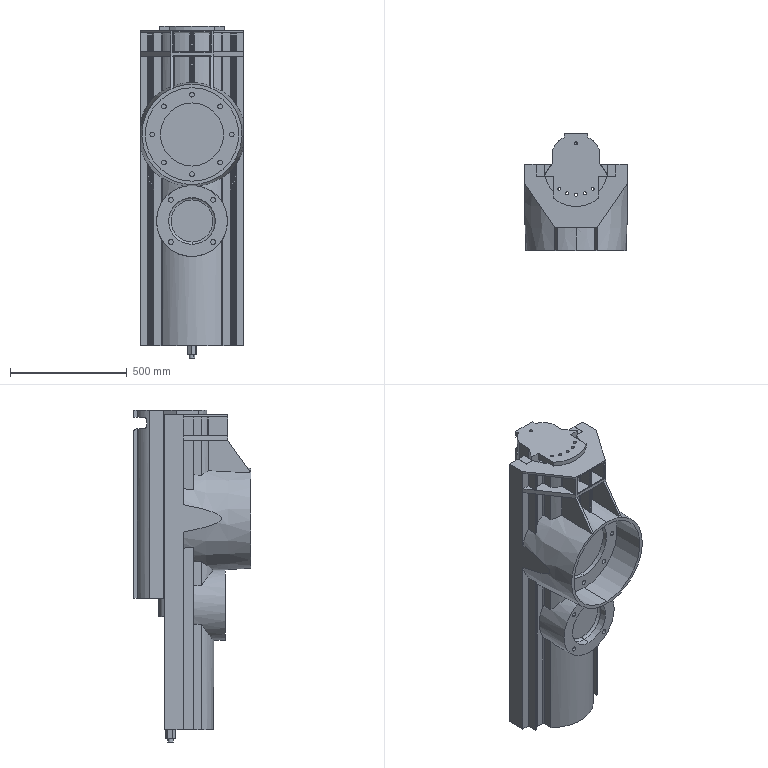Part | SolidWorks | 34 solids | 1136 faces | box 440 x 501.037 x 1420 mm | volume 76024148 mm3 | plane 626 | cylinder 343 | cone 117 | torus 50 | commonest cylinder face diameters 10 x77 16 x66 26 x42 14 x32 20 x24 4 x22